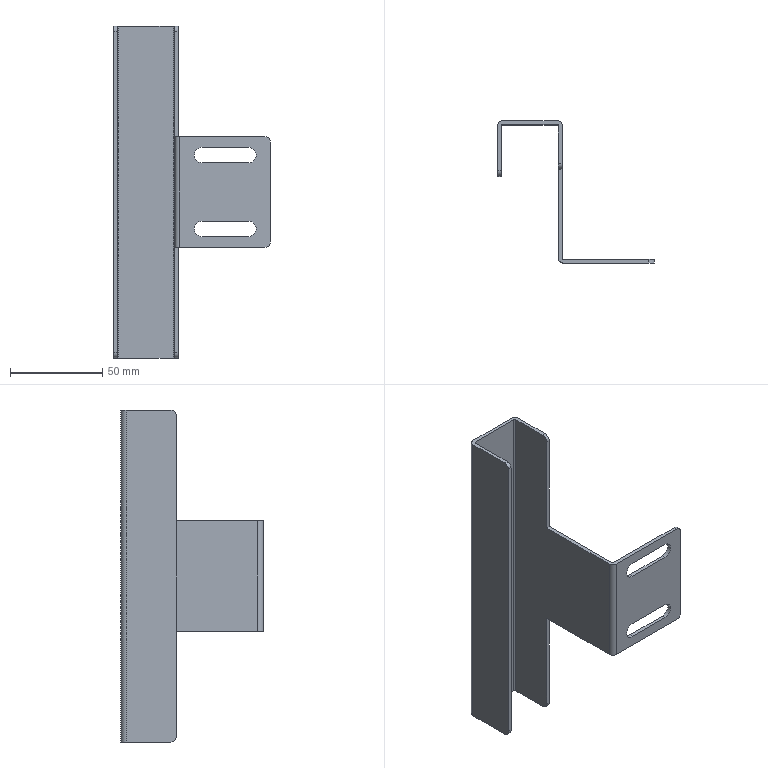Part | SolidWorks | features BaseBody 1 | 1 solid | 36 faces | box 85 x 77 x 180 mm | volume 41775 mm3 | plane 20 | cylinder 16 | commonest cylinder face diameters 6 x6 8.5 x4 1.473 x3 5.473 x3
STEP:
#1=CARTESIAN_POINT('',(35.,-23.255,-90.));
#2=VERTEX_POINT('',#1);
#3=CARTESIAN_POINT('',(35.,-2.737,-90.));
#4=VERTEX_POINT('',#3);
#5=CARTESIAN_POINT('',(35.,0.,-90.));
#6=DIRECTION('',(0.,1.,0.));
#7=VECTOR('',#6,1000.);
#8=LINE('',#5,#7);
#9=EDGE_CURVE('',#2,#4,#8,.T.);
#10=ORIENTED_EDGE('',*,*,#9,.T.);
#11=CARTESIAN_POINT('',(35.,-2.737,90.));
#12=VERTEX_POINT('',#11);
#13=CARTESIAN_POINT('',(35.,-2.737,90.));
#14=DIRECTION('',(0.,0.,1.));
#15=VECTOR('',#14,1000.);
#16=LINE('',#13,#15);
#17=EDGE_CURVE('',#4,#12,#16,.T.);
#18=ORIENTED_EDGE('',*,*,#17,.T.);
#19=CARTESIAN_POINT('',(35.,-23.255,90.));
#20=VERTEX_POINT('',#19);
#21=CARTESIAN_POINT('',(35.,0.,90.));
#22=DIRECTION('',(0.,-1.,0.));
#23=VECTOR('',#22,1000.);
#24=LINE('',#21,#23);
#25=EDGE_CURVE('',#12,#20,#24,.T.);
#26=ORIENTED_EDGE('',*,*,#25,.T.);
#27=CARTESIAN_POINT('',(35.,-26.255,87.));
#28=VERTEX_POINT('',#27);
#29=CARTESIAN_POINT('',(35.,-23.255,87.));
#30=DIRECTION('',(1.,0.,0.));
#31=DIRECTION('',(0.,0.,1.));
#32=AXIS2_PLACEMENT_3D('',#29,#30,#31);
#33=CIRCLE('',#32,3.);
#34=EDGE_CURVE('',#20,#28,#33,.T.);
#35=ORIENTED_EDGE('',*,*,#34,.T.);
#36=CARTESIAN_POINT('',(35.,-26.255,30.));
#37=VERTEX_POINT('',#36);
#38=CARTESIAN_POINT('',(35.,-26.255,90.));
#39=DIRECTION('',(0.,0.,-1.));
#40=VECTOR('',#39,1000.);
#41=LINE('',#38,#40);
#42=EDGE_CURVE('',#28,#37,#41,.T.);
#43=ORIENTED_EDGE('',*,*,#42,.T.);
#44=CARTESIAN_POINT('',(35.,-74.263,30.));
#45=VERTEX_POINT('',#44);
#46=CARTESIAN_POINT('',(35.,0.,30.));
#47=DIRECTION('',(0.,-1.,0.));
#48=VECTOR('',#47,1000.);
#49=LINE('',#46,#48);
#50=EDGE_CURVE('',#37,#45,#49,.T.);
#51=ORIENTED_EDGE('',*,*,#50,.T.);
#52=CARTESIAN_POINT('',(35.,-74.263,-30.));
#53=VERTEX_POINT('',#52);
#54=CARTESIAN_POINT('',(35.,-74.263,90.));
#55=DIRECTION('',(0.,0.,-1.));
#56=VECTOR('',#55,1000.);
#57=LINE('',#54,#56);
#58=EDGE_CURVE('',#45,#53,#57,.T.);
#59=ORIENTED_EDGE('',*,*,#58,.T.);
#60=CARTESIAN_POINT('',(35.,-26.255,-30.));
#61=VERTEX_POINT('',#60);
#62=CARTESIAN_POINT('',(35.,0.,-30.));
#63=DIRECTION('',(0.,1.,0.));
#64=VECTOR('',#63,1000.);
#65=LINE('',#62,#64);
#66=EDGE_CURVE('',#53,#61,#65,.T.);
#67=ORIENTED_EDGE('',*,*,#66,.T.);
#68=CARTESIAN_POINT('',(35.,-26.255,-87.));
#69=VERTEX_POINT('',#68);
#70=CARTESIAN_POINT('',(35.,-26.255,90.));
#71=DIRECTION('',(0.,0.,-1.));
#72=VECTOR('',#71,1000.);
#73=LINE('',#70,#72);
#74=EDGE_CURVE('',#61,#69,#73,.T.);
#75=ORIENTED_EDGE('',*,*,#74,.T.);
#76=CARTESIAN_POINT('',(35.,-23.255,-87.));
#77=DIRECTION('',(1.,0.,0.));
#78=DIRECTION('',(0.,0.,1.));
#79=AXIS2_PLACEMENT_3D('',#76,#77,#78);
#80=CIRCLE('',#79,3.);
#81=EDGE_CURVE('',#69,#2,#80,.T.);
#82=ORIENTED_EDGE('',*,*,#81,.T.);
#83=EDGE_LOOP('',(#10,#18,#26,#35,#43,#51,#59,#67,#75,#82));
#84=FACE_OUTER_BOUND('',#83,.T.);
#85=CARTESIAN_POINT('',(35.,0.,90.));
#86=DIRECTION('',(1.,0.,0.));
#87=DIRECTION('',(0.,0.,-1.));
#88=AXIS2_PLACEMENT_3D('',#85,#86,#87);
#89=PLANE('',#88);
#90=ADVANCED_FACE('',(#84),#89,.T.);
#91=CARTESIAN_POINT('',(32.263,0.,90.));
#92=VERTEX_POINT('',#91);
#93=CARTESIAN_POINT('',(32.263,-2.737,90.));
#94=DIRECTION('',(0.,0.,-1.));
#95=DIRECTION('',(-1.,0.,0.));
#96=AXIS2_PLACEMENT_3D('',#93,#94,#95);
#97=CIRCLE('',#96,2.737);
#98=EDGE_CURVE('',#92,#12,#97,.T.);
#99=ORIENTED_EDGE('',*,*,#98,.T.);
#100=ORIENTED_EDGE('',*,*,#17,.F.);
#101=CARTESIAN_POINT('',(32.263,0.,-90.));
#102=VERTEX_POINT('',#101);
#103=CARTESIAN_POINT('',(32.263,-2.737,-90.));
#104=DIRECTION('',(0.,0.,1.));
#105=DIRECTION('',(-1.,0.,0.));
#106=AXIS2_PLACEMENT_3D('',#103,#104,#105);
#107=CIRCLE('',#106,2.737);
#108=EDGE_CURVE('',#4,#102,#107,.T.);
#109=ORIENTED_EDGE('',*,*,#108,.T.);
#110=CARTESIAN_POINT('',(32.263,0.,90.));
#111=DIRECTION('',(0.,0.,1.));
#112=VECTOR('',#111,1000.);
#113=LINE('',#110,#112);
#114=EDGE_CURVE('',#102,#92,#113,.T.);
#115=ORIENTED_EDGE('',*,*,#114,.T.);
#116=EDGE_LOOP('',(#99,#100,#109,#115));
#117=FACE_OUTER_BOUND('',#116,.T.);
#118=CARTESIAN_POINT('',(32.263,-2.737,90.));
#119=DIRECTION('',(0.,0.,-1.));
#120=DIRECTION('',(-1.,0.,0.));
#121=AXIS2_PLACEMENT_3D('',#118,#119,#120);
#122=CYLINDRICAL_SURFACE('',#121,2.737);
#123=ADVANCED_FACE('',(#117),#122,.T.);
#124=CARTESIAN_POINT('',(33.,-23.255,-90.));
#125=VERTEX_POINT('',#124);
#126=CARTESIAN_POINT('',(33.,-2.737,-90.));
#127=VERTEX_POINT('',#126);
#128=CARTESIAN_POINT('',(33.,-77.,-90.));
#129=DIRECTION('',(0.,1.,0.));
#130=VECTOR('',#129,1000.);
#131=LINE('',#128,#130);
#132=EDGE_CURVE('',#125,#127,#131,.T.);
#133=ORIENTED_EDGE('',*,*,#132,.T.);
#134=CARTESIAN_POINT('',(32.263,-2.,-90.));
#135=VERTEX_POINT('',#134);
#136=CARTESIAN_POINT('',(32.263,-2.737,-90.));
#137=DIRECTION('',(0.,0.,1.));
#138=DIRECTION('',(-1.,0.,0.));
#139=AXIS2_PLACEMENT_3D('',#136,#137,#138);
#140=CIRCLE('',#139,0.7366);
#141=EDGE_CURVE('',#127,#135,#140,.T.);
#142=ORIENTED_EDGE('',*,*,#141,.T.);
#143=CARTESIAN_POINT('',(2.737,-2.,-90.));
#144=VERTEX_POINT('',#143);
#145=CARTESIAN_POINT('',(33.,-2.,-90.));
#146=DIRECTION('',(-1.,0.,0.));
#147=VECTOR('',#146,1000.);
#148=LINE('',#145,#147);
#149=EDGE_CURVE('',#135,#144,#148,.T.);
#150=ORIENTED_EDGE('',*,*,#149,.T.);
#151=CARTESIAN_POINT('',(2.,-2.737,-90.));
#152=VERTEX_POINT('',#151);
#153=CARTESIAN_POINT('',(2.737,-2.737,-90.));
#154=DIRECTION('',(0.,0.,1.));
#155=DIRECTION('',(-1.,0.,0.));
#156=AXIS2_PLACEMENT_3D('',#153,#154,#155);
#157=CIRCLE('',#156,0.7366);
#158=EDGE_CURVE('',#144,#152,#157,.T.);
#159=ORIENTED_EDGE('',*,*,#158,.T.);
#160=CARTESIAN_POINT('',(2.,-27.,-90.));
#161=VERTEX_POINT('',#160);
#162=CARTESIAN_POINT('',(2.,-2.,-90.));
#163=DIRECTION('',(0.,-1.,0.));
#164=VECTOR('',#163,1000.);
#165=LINE('',#162,#164);
#166=EDGE_CURVE('',#152,#161,#165,.T.);
#167=ORIENTED_EDGE('',*,*,#166,.T.);
#168=CARTESIAN_POINT('',(0.,-27.,-90.));
#169=VERTEX_POINT('',#168);
#170=CARTESIAN_POINT('',(2.737,-27.,-90.));
#171=DIRECTION('',(1.,0.,0.));
#172=VECTOR('',#171,1000.);
#173=LINE('',#170,#172);
#174=EDGE_CURVE('',#169,#161,#173,.T.);
#175=ORIENTED_EDGE('',*,*,#174,.F.);
#176=CARTESIAN_POINT('',(0.,-2.737,-90.));
#177=VERTEX_POINT('',#176);
#178=CARTESIAN_POINT('',(0.,-30.,-90.));
#179=DIRECTION('',(0.,-1.,0.));
#180=VECTOR('',#179,1000.);
#181=LINE('',#178,#180);
#182=EDGE_CURVE('',#177,#169,#181,.T.);
#183=ORIENTED_EDGE('',*,*,#182,.F.);
#184=CARTESIAN_POINT('',(2.737,0.,-90.));
#185=VERTEX_POINT('',#184);
#186=CARTESIAN_POINT('',(2.737,-2.737,-90.));
#187=DIRECTION('',(0.,0.,1.));
#188=DIRECTION('',(-1.,0.,0.));
#189=AXIS2_PLACEMENT_3D('',#186,#187,#188);
#190=CIRCLE('',#189,2.737);
#191=EDGE_CURVE('',#185,#177,#190,.T.);
#192=ORIENTED_EDGE('',*,*,#191,.F.);
#193=CARTESIAN_POINT('',(0.,0.,-90.));
#194=DIRECTION('',(-1.,0.,0.));
#195=VECTOR('',#194,1000.);
#196=LINE('',#193,#195);
#197=EDGE_CURVE('',#102,#185,#196,.T.);
#198=ORIENTED_EDGE('',*,*,#197,.F.);
#199=ORIENTED_EDGE('',*,*,#108,.F.);
#200=ORIENTED_EDGE('',*,*,#9,.F.);
#201=CARTESIAN_POINT('',(35.737,-23.255,-90.));
#202=DIRECTION('',(-1.,0.,0.));
#203=VECTOR('',#202,1000.);
#204=LINE('',#201,#203);
#205=EDGE_CURVE('',#2,#125,#204,.T.);
#206=ORIENTED_EDGE('',*,*,#205,.T.);
#207=EDGE_LOOP('',(#133,#142,#150,#159,#167,#175,#183,#192,#198,#199,#200,#206));
#208=FACE_OUTER_BOUND('',#207,.T.);
#209=CARTESIAN_POINT('',(35.737,-77.,-90.));
#210=DIRECTION('',(0.,0.,-1.));
#211=DIRECTION('',(-1.,0.,0.));
#212=AXIS2_PLACEMENT_3D('',#209,#210,#211);
#213=PLANE('',#212);
#214=ADVANCED_FACE('',(#208),#213,.T.);
#215=ORIENTED_EDGE('',*,*,#81,.F.);
#216=CARTESIAN_POINT('',(33.,-26.255,-87.));
#217=VERTEX_POINT('',#216);
#218=CARTESIAN_POINT('',(25.,-26.255,-87.));
#219=DIRECTION('',(-1.,0.,0.));
#220=VECTOR('',#219,1000.);
#221=LINE('',#218,#220);
#222=EDGE_CURVE('',#69,#217,#221,.T.);
#223=ORIENTED_EDGE('',*,*,#222,.T.);
#224=CARTESIAN_POINT('',(33.,-23.255,-87.));
#225=DIRECTION('',(1.,0.,0.));
#226=DIRECTION('',(0.,0.,1.));
#227=AXIS2_PLACEMENT_3D('',#224,#225,#226);
#228=CIRCLE('',#227,3.);
#229=EDGE_CURVE('',#217,#125,#228,.T.);
#230=ORIENTED_EDGE('',*,*,#229,.T.);
#231=ORIENTED_EDGE('',*,*,#205,.F.);
#232=EDGE_LOOP('',(#215,#223,#230,#231));
#233=FACE_OUTER_BOUND('',#232,.T.);
#234=CARTESIAN_POINT('',(25.,-23.255,-87.));
#235=DIRECTION('',(-1.,0.,0.));
#236=DIRECTION('',(0.,0.,1.));
#237=AXIS2_PLACEMENT_3D('',#234,#235,#236);
#238=CYLINDRICAL_SURFACE('',#237,3.);
#239=ADVANCED_FACE('',(#233),#238,.T.);
#240=ORIENTED_EDGE('',*,*,#222,.F.);
#241=ORIENTED_EDGE('',*,*,#74,.F.);
#242=CARTESIAN_POINT('',(33.,-26.255,-30.));
#243=VERTEX_POINT('',#242);
#244=CARTESIAN_POINT('',(25.,-26.255,-30.));
#245=DIRECTION('',(1.,0.,0.));
#246=VECTOR('',#245,1000.);
#247=LINE('',#244,#246);
#248=EDGE_CURVE('',#243,#61,#247,.T.);
#249=ORIENTED_EDGE('',*,*,#248,.F.);
#250=CARTESIAN_POINT('',(33.,-26.255,-90.));
#251=DIRECTION('',(0.,0.,1.));
#252=VECTOR('',#251,1000.);
#253=LINE('',#250,#252);
#254=EDGE_CURVE('',#217,#243,#253,.T.);
#255=ORIENTED_EDGE('',*,*,#254,.F.);
#256=EDGE_LOOP('',(#240,#241,#249,#255));
#257=FACE_OUTER_BOUND('',#256,.T.);
#258=CARTESIAN_POINT('',(25.,-26.255,-90.));
#259=DIRECTION('',(0.,1.,0.));
#260=DIRECTION('',(0.,0.,1.));
#261=AXIS2_PLACEMENT_3D('',#258,#259,#260);
#262=PLANE('',#261);
#263=ADVANCED_FACE('',(#257),#262,.F.);
#264=CARTESIAN_POINT('',(33.,-74.263,-30.));
#265=VERTEX_POINT('',#264);
#266=CARTESIAN_POINT('',(33.,-126.255,-30.));
#267=DIRECTION('',(0.,-1.,0.));
#268=VECTOR('',#267,1000.);
#269=LINE('',#266,#268);
#270=EDGE_CURVE('',#243,#265,#269,.T.);
#271=ORIENTED_EDGE('',*,*,#270,.F.);
#272=ORIENTED_EDGE('',*,*,#248,.T.);
#273=ORIENTED_EDGE('',*,*,#66,.F.);
#274=CARTESIAN_POINT('',(35.737,-75.,-30.));
#275=VERTEX_POINT('',#274);
#276=CARTESIAN_POINT('',(35.737,-74.263,-30.));
#277=DIRECTION('',(0.,0.,1.));
#278=DIRECTION('',(-1.,0.,0.));
#279=AXIS2_PLACEMENT_3D('',#276,#277,#278);
#280=CIRCLE('',#279,0.7366);
#281=EDGE_CURVE('',#53,#275,#280,.T.);
#282=ORIENTED_EDGE('',*,*,#281,.T.);
#283=CARTESIAN_POINT('',(82.,-75.,-30.));
#284=VERTEX_POINT('',#283);
#285=CARTESIAN_POINT('',(35.,-75.,-30.));
#286=DIRECTION('',(-1.,0.,0.));
#287=VECTOR('',#286,1000.);
#288=LINE('',#285,#287);
#289=EDGE_CURVE('',#284,#275,#288,.T.);
#290=ORIENTED_EDGE('',*,*,#289,.F.);
#291=CARTESIAN_POINT('',(82.,-77.,-30.));
#292=VERTEX_POINT('',#291);
#293=CARTESIAN_POINT('',(82.,-85.,-30.));
#294=DIRECTION('',(0.,1.,0.));
#295=VECTOR('',#294,1000.);
#296=LINE('',#293,#295);
#297=EDGE_CURVE('',#292,#284,#296,.T.);
#298=ORIENTED_EDGE('',*,*,#297,.F.);
#299=CARTESIAN_POINT('',(35.737,-77.,-30.));
#300=VERTEX_POINT('',#299);
#301=CARTESIAN_POINT('',(85.,-77.,-30.));
#302=DIRECTION('',(1.,0.,0.));
#303=VECTOR('',#302,1000.);
#304=LINE('',#301,#303);
#305=EDGE_CURVE('',#300,#292,#304,.T.);
#306=ORIENTED_EDGE('',*,*,#305,.F.);
#307=CARTESIAN_POINT('',(35.737,-74.263,-30.));
#308=DIRECTION('',(0.,0.,1.));
#309=DIRECTION('',(-1.,0.,0.));
#310=AXIS2_PLACEMENT_3D('',#307,#308,#309);
#311=CIRCLE('',#310,2.737);
#312=EDGE_CURVE('',#265,#300,#311,.T.);
#313=ORIENTED_EDGE('',*,*,#312,.F.);
#314=EDGE_LOOP('',(#271,#272,#273,#282,#290,#298,#306,#313));
#315=FACE_OUTER_BOUND('',#314,.T.);
#316=CARTESIAN_POINT('',(25.,-126.255,-30.));
#317=DIRECTION('',(0.,0.,1.));
#318=DIRECTION('',(1.,0.,0.));
#319=AXIS2_PLACEMENT_3D('',#316,#317,#318);
#320=PLANE('',#319);
#321=ADVANCED_FACE('',(#315),#320,.F.);
#322=ORIENTED_EDGE('',*,*,#58,.F.);
#323=CARTESIAN_POINT('',(35.737,-75.,30.));
#324=VERTEX_POINT('',#323);
#325=CARTESIAN_POINT('',(35.737,-74.263,30.));
#326=DIRECTION('',(0.,0.,1.));
#327=DIRECTION('',(-1.,0.,0.));
#328=AXIS2_PLACEMENT_3D('',#325,#326,#327);
#329=CIRCLE('',#328,0.7366);
#330=EDGE_CURVE('',#45,#324,#329,.T.);
#331=ORIENTED_EDGE('',*,*,#330,.T.);
#332=CARTESIAN_POINT('',(35.737,-75.,60.095));
#333=DIRECTION('',(0.,0.,1.));
#334=VECTOR('',#333,1000.);
#335=LINE('',#332,#334);
#336=EDGE_CURVE('',#275,#324,#335,.T.);
#337=ORIENTED_EDGE('',*,*,#336,.F.);
#338=ORIENTED_EDGE('',*,*,#281,.F.);
#339=EDGE_LOOP('',(#322,#331,#337,#338));
#340=FACE_OUTER_BOUND('',#339,.T.);
#341=CARTESIAN_POINT('',(35.737,-74.263,60.095));
#342=DIRECTION('',(0.,0.,-1.));
#343=DIRECTION('',(-1.,0.,0.));
#344=AXIS2_PLACEMENT_3D('',#341,#342,#343);
#345=CYLINDRICAL_SURFACE('',#344,0.7366);
#346=ADVANCED_FACE('',(#340),#345,.F.);
#347=ORIENTED_EDGE('',*,*,#50,.F.);
#348=CARTESIAN_POINT('',(33.,-26.255,30.));
#349=VERTEX_POINT('',#348);
#350=CARTESIAN_POINT('',(25.,-26.255,30.));
#351=DIRECTION('',(1.,0.,0.));
#352=VECTOR('',#351,1000.);
#353=LINE('',#350,#352);
#354=EDGE_CURVE('',#349,#37,#353,.T.);
#355=ORIENTED_EDGE('',*,*,#354,.F.);
#356=CARTESIAN_POINT('',(33.,-74.263,30.));
#357=VERTEX_POINT('',#356);
#358=CARTESIAN_POINT('',(33.,-126.255,30.));
#359=DIRECTION('',(0.,1.,0.));
#360=VECTOR('',#359,1000.);
#361=LINE('',#358,#360);
#362=EDGE_CURVE('',#357,#349,#361,.T.);
#363=ORIENTED_EDGE('',*,*,#362,.F.);
#364=CARTESIAN_POINT('',(35.737,-77.,30.));
#365=VERTEX_POINT('',#364);
#366=CARTESIAN_POINT('',(35.737,-74.263,30.));
#367=DIRECTION('',(0.,0.,-1.));
#368=DIRECTION('',(-1.,0.,0.));
#369=AXIS2_PLACEMENT_3D('',#366,#367,#368);
#370=CIRCLE('',#369,2.737);
#371=EDGE_CURVE('',#365,#357,#370,.T.);
#372=ORIENTED_EDGE('',*,*,#371,.F.);
#373=CARTESIAN_POINT('',(82.,-77.,30.));
#374=VERTEX_POINT('',#373);
#375=CARTESIAN_POINT('',(85.,-77.,30.));
#376=DIRECTION('',(-1.,0.,0.));
#377=VECTOR('',#376,1000.);
#378=LINE('',#375,#377);
#379=EDGE_CURVE('',#374,#365,#378,.T.);
#380=ORIENTED_EDGE('',*,*,#379,.F.);
#381=CARTESIAN_POINT('',(82.,-75.,30.));
#382=VERTEX_POINT('',#381);
#383=CARTESIAN_POINT('',(82.,-85.,30.));
#384=DIRECTION('',(0.,-1.,0.));
#385=VECTOR('',#384,1000.);
#386=LINE('',#383,#385);
#387=EDGE_CURVE('',#382,#374,#386,.T.);
#388=ORIENTED_EDGE('',*,*,#387,.F.);
#389=CARTESIAN_POINT('',(35.,-75.,30.));
#390=DIRECTION('',(1.,0.,0.));
#391=VECTOR('',#390,1000.);
#392=LINE('',#389,#391);
#393=EDGE_CURVE('',#324,#382,#392,.T.);
#394=ORIENTED_EDGE('',*,*,#393,.F.);
#395=ORIENTED_EDGE('',*,*,#330,.F.);
#396=EDGE_LOOP('',(#347,#355,#363,#372,#380,#388,#394,#395));
#397=FACE_OUTER_BOUND('',#396,.T.);
#398=CARTESIAN_POINT('',(25.,-126.255,30.));
#399=DIRECTION('',(0.,0.,-1.));
#400=DIRECTION('',(0.,1.,0.));
#401=AXIS2_PLACEMENT_3D('',#398,#399,#400);
#402=PLANE('',#401);
#403=ADVANCED_FACE('',(#397),#402,.F.);
#404=CARTESIAN_POINT('',(33.,-26.255,87.));
#405=VERTEX_POINT('',#404);
#406=CARTESIAN_POINT('',(25.,-26.255,87.));
#407=DIRECTION('',(1.,0.,0.));
#408=VECTOR('',#407,1000.);
#409=LINE('',#406,#408);
#410=EDGE_CURVE('',#405,#28,#409,.T.);
#411=ORIENTED_EDGE('',*,*,#410,.F.);
#412=CARTESIAN_POINT('',(33.,-26.255,90.));
#413=DIRECTION('',(0.,0.,1.));
#414=VECTOR('',#413,1000.);
#415=LINE('',#412,#414);
#416=EDGE_CURVE('',#349,#405,#415,.T.);
#417=ORIENTED_EDGE('',*,*,#416,.F.);
#418=ORIENTED_EDGE('',*,*,#354,.T.);
#419=ORIENTED_EDGE('',*,*,#42,.F.);
#420=EDGE_LOOP('',(#411,#417,#418,#419));
#421=FACE_OUTER_BOUND('',#420,.T.);
#422=CARTESIAN_POINT('',(25.,-26.255,90.));
#423=DIRECTION('',(0.,1.,0.));
#424=DIRECTION('',(0.,0.,1.));
#425=AXIS2_PLACEMENT_3D('',#422,#423,#424);
#426=PLANE('',#425);
#427=ADVANCED_FACE('',(#421),#426,.F.);
#428=ORIENTED_EDGE('',*,*,#34,.F.);
#429=CARTESIAN_POINT('',(33.,-23.255,90.));
#430=VERTEX_POINT('',#429);
#431=CARTESIAN_POINT('',(32.263,-23.255,90.));
#432=DIRECTION('',(-1.,0.,0.));
#433=VECTOR('',#432,1000.);
#434=LINE('',#431,#433);
#435=EDGE_CURVE('',#20,#430,#434,.T.);
#436=ORIENTED_EDGE('',*,*,#435,.T.);
#437=CARTESIAN_POINT('',(33.,-23.255,87.));
#438=DIRECTION('',(1.,0.,0.));
#439=DIRECTION('',(0.,0.,1.));
#440=AXIS2_PLACEMENT_3D('',#437,#438,#439);
#441=CIRCLE('',#440,3.);
#442=EDGE_CURVE('',#430,#405,#441,.T.);
#443=ORIENTED_EDGE('',*,*,#442,.T.);
#444=ORIENTED_EDGE('',*,*,#410,.T.);
#445=EDGE_LOOP('',(#428,#436,#443,#444));
#446=FACE_OUTER_BOUND('',#445,.T.);
#447=CARTESIAN_POINT('',(32.263,-23.255,87.));
#448=DIRECTION('',(-1.,0.,0.));
#449=DIRECTION('',(0.,0.,1.));
#450=AXIS2_PLACEMENT_3D('',#447,#448,#449);
#451=CYLINDRICAL_SURFACE('',#450,3.);
#452=ADVANCED_FACE('',(#446),#451,.T.);
#453=ORIENTED_EDGE('',*,*,#25,.F.);
#454=ORIENTED_EDGE('',*,*,#98,.F.);
#455=CARTESIAN_POINT('',(2.737,0.,90.));
#456=VERTEX_POINT('',#455);
#457=CARTESIAN_POINT('',(0.,0.,90.));
#458=DIRECTION('',(1.,0.,0.));
#459=VECTOR('',#458,1000.);
#460=LINE('',#457,#459);
#461=EDGE_CURVE('',#456,#92,#460,.T.);
#462=ORIENTED_EDGE('',*,*,#461,.F.);
#463=CARTESIAN_POINT('',(0.,-2.737,90.));
#464=VERTEX_POINT('',#463);
#465=CARTESIAN_POINT('',(2.737,-2.737,90.));
#466=DIRECTION('',(0.,0.,-1.));
#467=DIRECTION('',(-1.,0.,0.));
#468=AXIS2_PLACEMENT_3D('',#465,#466,#467);
#469=CIRCLE('',#468,2.737);
#470=EDGE_CURVE('',#464,#456,#469,.T.);
#471=ORIENTED_EDGE('',*,*,#470,.F.);
#472=CARTESIAN_POINT('',(0.,-27.,90.));
#473=VERTEX_POINT('',#472);
#474=CARTESIAN_POINT('',(0.,-30.,90.));
#475=DIRECTION('',(0.,1.,0.));
#476=VECTOR('',#475,1000.);
#477=LINE('',#474,#476);
#478=EDGE_CURVE('',#473,#464,#477,.T.);
#479=ORIENTED_EDGE('',*,*,#478,.F.);
#480=CARTESIAN_POINT('',(2.,-27.,90.));
#481=VERTEX_POINT('',#480);
#482=CARTESIAN_POINT('',(35.737,-27.,90.));
#483=DIRECTION('',(-1.,0.,0.));
#484=VECTOR('',#483,1000.);
#485=LINE('',#482,#484);
#486=EDGE_CURVE('',#481,#473,#485,.T.);
#487=ORIENTED_EDGE('',*,*,#486,.F.);
#488=CARTESIAN_POINT('',(2.,-2.737,90.));
#489=VERTEX_POINT('',#488);
#490=CARTESIAN_POINT('',(2.,-74.263,90.));
#491=DIRECTION('',(0.,-1.,0.));
#492=VECTOR('',#491,1000.);
#493=LINE('',#490,#492);
#494=EDGE_CURVE('',#489,#481,#493,.T.);
#495=ORIENTED_EDGE('',*,*,#494,.F.);
#496=CARTESIAN_POINT('',(2.737,-2.,90.));
#497=VERTEX_POINT('',#496);
#498=CARTESIAN_POINT('',(2.737,-2.737,90.));
#499=DIRECTION('',(0.,0.,-1.));
#500=DIRECTION('',(-1.,0.,0.));
#501=AXIS2_PLACEMENT_3D('',#498,#499,#500);
#502=CIRCLE('',#501,0.7366);
#503=EDGE_CURVE('',#489,#497,#502,.T.);
#504=ORIENTED_EDGE('',*,*,#503,.T.);
#505=CARTESIAN_POINT('',(32.263,-2.,90.));
#506=VERTEX_POINT('',#505);
#507=CARTESIAN_POINT('',(2.,-2.,90.));
#508=DIRECTION('',(1.,0.,0.));
#509=VECTOR('',#508,1000.);
#510=LINE('',#507,#509);
#511=EDGE_CURVE('',#497,#506,#510,.T.);
#512=ORIENTED_EDGE('',*,*,#511,.T.);
#513=CARTESIAN_POINT('',(33.,-2.737,90.));
#514=VERTEX_POINT('',#513);
#515=CARTESIAN_POINT('',(32.263,-2.737,90.));
#516=DIRECTION('',(0.,0.,-1.));
#517=DIRECTION('',(-1.,0.,0.));
#518=AXIS2_PLACEMENT_3D('',#515,#516,#517);
#519=CIRCLE('',#518,0.7366);
#520=EDGE_CURVE('',#506,#514,#519,.T.);
#521=ORIENTED_EDGE('',*,*,#520,.T.);
#522=CARTESIAN_POINT('',(33.,-2.,90.));
#523=DIRECTION('',(0.,-1.,0.));
#524=VECTOR('',#523,1000.);
#525=LINE('',#522,#524);
#526=EDGE_CURVE('',#514,#430,#525,.T.);
#527=ORIENTED_EDGE('',*,*,#526,.T.);
#528=ORIENTED_EDGE('',*,*,#435,.F.);
#529=EDGE_LOOP('',(#453,#454,#462,#471,#479,#487,#495,#504,#512,#521,#527,#528));
#530=FACE_OUTER_BOUND('',#529,.T.);
#531=CARTESIAN_POINT('',(32.263,-2.,90.));
#532=DIRECTION('',(0.,0.,1.));
#533=DIRECTION('',(1.,0.,0.));
#534=AXIS2_PLACEMENT_3D('',#531,#532,#533);
#535=PLANE('',#534);
#536=ADVANCED_FACE('',(#530),#535,.T.);
#537=ORIENTED_EDGE('',*,*,#461,.T.);
#538=ORIENTED_EDGE('',*,*,#114,.F.);
#539=ORIENTED_EDGE('',*,*,#197,.T.);
#540=CARTESIAN_POINT('',(2.737,0.,90.));
#541=DIRECTION('',(0.,0.,1.));
#542=VECTOR('',#541,1000.);
#543=LINE('',#540,#542);
#544=EDGE_CURVE('',#185,#456,#543,.T.);
#545=ORIENTED_EDGE('',*,*,#544,.T.);
#546=EDGE_LOOP('',(#537,#538,#539,#545));
#547=FACE_OUTER_BOUND('',#546,.T.);
#548=CARTESIAN_POINT('',(0.,0.,90.));
#549=DIRECTION('',(0.,1.,0.));
#550=DIRECTION('',(0.,0.,1.));
#551=AXIS2_PLACEMENT_3D('',#548,#549,#550);
#552=PLANE('',#551);
#553=ADVANCED_FACE('',(#547),#552,.T.);
#554=ORIENTED_EDGE('',*,*,#442,.F.);
#555=ORIENTED_EDGE('',*,*,#526,.F.);
#556=CARTESIAN_POINT('',(33.,-2.737,90.));
#557=DIRECTION('',(0.,0.,1.));
#558=VECTOR('',#557,1000.);
#559=LINE('',#556,#558);
#560=EDGE_CURVE('',#127,#514,#559,.T.);
#561=ORIENTED_EDGE('',*,*,#560,.F.);
#562=ORIENTED_EDGE('',*,*,#132,.F.);
#563=ORIENTED_EDGE('',*,*,#229,.F.);
#564=ORIENTED_EDGE('',*,*,#254,.T.);
#565=ORIENTED_EDGE('',*,*,#270,.T.);
#566=CARTESIAN_POINT('',(33.,-74.263,90.));
#567=DIRECTION('',(0.,0.,-1.));
#568=VECTOR('',#567,1000.);
#569=LINE('',#566,#568);
#570=EDGE_CURVE('',#357,#265,#569,.T.);
#571=ORIENTED_EDGE('',*,*,#570,.F.);
#572=ORIENTED_EDGE('',*,*,#362,.T.);
#573=ORIENTED_EDGE('',*,*,#416,.T.);
#574=EDGE_LOOP('',(#554,#555,#561,#562,#563,#564,#565,#571,#572,#573));
#575=FACE_OUTER_BOUND('',#574,.T.);
#576=CARTESIAN_POINT('',(33.,0.,90.));
#577=DIRECTION('',(1.,0.,0.));
#578=DIRECTION('',(0.,0.,-1.));
#579=AXIS2_PLACEMENT_3D('',#576,#577,#578);
#580=PLANE('',#579);
#581=ADVANCED_FACE('',(#575),#580,.F.);
#582=ORIENTED_EDGE('',*,*,#393,.T.);
#583=CARTESIAN_POINT('',(85.,-75.,27.));
#584=VERTEX_POINT('',#583);
#585=CARTESIAN_POINT('',(82.,-75.,27.));
#586=DIRECTION('',(0.,1.,0.));
#587=DIRECTION('',(0.,0.,-1.));
#588=AXIS2_PLACEMENT_3D('',#585,#586,#587);
#589=CIRCLE('',#588,3.);
#590=EDGE_CURVE('',#382,#584,#589,.T.);
#591=ORIENTED_EDGE('',*,*,#590,.T.);
#592=CARTESIAN_POINT('',(85.,-75.,-27.));
#593=VERTEX_POINT('',#592);
#594=CARTESIAN_POINT('',(85.,-75.,90.));
#595=DIRECTION('',(0.,0.,-1.));
#596=VECTOR('',#595,1000.);
#597=LINE('',#594,#596);
#598=EDGE_CURVE('',#584,#593,#597,.T.);
#599=ORIENTED_EDGE('',*,*,#598,.T.);
#600=CARTESIAN_POINT('',(82.,-75.,-27.));
#601=DIRECTION('',(0.,1.,0.));
#602=DIRECTION('',(0.,0.,-1.));
#603=AXIS2_PLACEMENT_3D('',#600,#601,#602);
#604=CIRCLE('',#603,3.);
#605=EDGE_CURVE('',#593,#284,#604,.T.);
#606=ORIENTED_EDGE('',*,*,#605,.T.);
#607=ORIENTED_EDGE('',*,*,#289,.T.);
#608=ORIENTED_EDGE('',*,*,#336,.T.);
#609=EDGE_LOOP('',(#582,#591,#599,#606,#607,#608));
#610=FACE_OUTER_BOUND('',#609,.T.);
#611=CARTESIAN_POINT('',(73.,-75.,15.75));
#612=VERTEX_POINT('',#611);
#613=CARTESIAN_POINT('',(73.,-75.,24.25));
#614=VERTEX_POINT('',#613);
#615=CARTESIAN_POINT('',(73.,-75.,20.));
#616=DIRECTION('',(0.,-1.,0.));
#617=DIRECTION('',(0.,0.,1.));
#618=AXIS2_PLACEMENT_3D('',#615,#616,#617);
#619=CIRCLE('',#618,4.25);
#620=EDGE_CURVE('',#612,#614,#619,.T.);
#621=ORIENTED_EDGE('',*,*,#620,.T.);
#622=CARTESIAN_POINT('',(48.,-75.,24.25));
#623=VERTEX_POINT('',#622);
#624=CARTESIAN_POINT('',(35.,-75.,24.25));
#625=DIRECTION('',(-1.,0.,0.));
#626=VECTOR('',#625,1000.);
#627=LINE('',#624,#626);
#628=EDGE_CURVE('',#614,#623,#627,.T.);
#629=ORIENTED_EDGE('',*,*,#628,.T.);
#630=CARTESIAN_POINT('',(48.,-75.,15.75));
#631=VERTEX_POINT('',#630);
#632=CARTESIAN_POINT('',(48.,-75.,20.));
#633=DIRECTION('',(0.,-1.,0.));
#634=DIRECTION('',(0.,0.,1.));
#635=AXIS2_PLACEMENT_3D('',#632,#633,#634);
#636=CIRCLE('',#635,4.25);
#637=EDGE_CURVE('',#623,#631,#636,.T.);
#638=ORIENTED_EDGE('',*,*,#637,.T.);
#639=CARTESIAN_POINT('',(35.,-75.,15.75));
#640=DIRECTION('',(1.,0.,0.));
#641=VECTOR('',#640,1000.);
#642=LINE('',#639,#641);
#643=EDGE_CURVE('',#631,#612,#642,.T.);
#644=ORIENTED_EDGE('',*,*,#643,.T.);
#645=EDGE_LOOP('',(#621,#629,#638,#644));
#646=FACE_BOUND('',#645,.T.);
#647=CARTESIAN_POINT('',(73.,-75.,-24.25));
#648=VERTEX_POINT('',#647);
#649=CARTESIAN_POINT('',(73.,-75.,-15.75));
#650=VERTEX_POINT('',#649);
#651=CARTESIAN_POINT('',(73.,-75.,-20.));
#652=DIRECTION('',(0.,-1.,0.));
#653=DIRECTION('',(0.,0.,1.));
#654=AXIS2_PLACEMENT_3D('',#651,#652,#653);
#655=CIRCLE('',#654,4.25);
#656=EDGE_CURVE('',#648,#650,#655,.T.);
#657=ORIENTED_EDGE('',*,*,#656,.T.);
#658=CARTESIAN_POINT('',(48.,-75.,-15.75));
#659=VERTEX_POINT('',#658);
#660=CARTESIAN_POINT('',(35.,-75.,-15.75));
#661=DIRECTION('',(-1.,0.,0.));
#662=VECTOR('',#661,1000.);
#663=LINE('',#660,#662);
#664=EDGE_CURVE('',#650,#659,#663,.T.);
#665=ORIENTED_EDGE('',*,*,#664,.T.);
#666=CARTESIAN_POINT('',(48.,-75.,-24.25));
#667=VERTEX_POINT('',#666);
#668=CARTESIAN_POINT('',(48.,-75.,-20.));
#669=DIRECTION('',(0.,-1.,0.));
#670=DIRECTION('',(0.,0.,1.));
#671=AXIS2_PLACEMENT_3D('',#668,#669,#670);
#672=CIRCLE('',#671,4.25);
#673=EDGE_CURVE('',#659,#667,#672,.T.);
#674=ORIENTED_EDGE('',*,*,#673,.T.);
#675=CARTESIAN_POINT('',(35.,-75.,-24.25));
#676=DIRECTION('',(1.,0.,0.));
#677=VECTOR('',#676,1000.);
#678=LINE('',#675,#677);
#679=EDGE_CURVE('',#667,#648,#678,.T.);
#680=ORIENTED_EDGE('',*,*,#679,.T.);
#681=EDGE_LOOP('',(#657,#665,#674,#680));
#682=FACE_BOUND('',#681,.T.);
#683=CARTESIAN_POINT('',(35.,-75.,90.));
#684=DIRECTION('',(0.,1.,0.));
#685=DIRECTION('',(0.,0.,1.));
#686=AXIS2_PLACEMENT_3D('',#683,#684,#685);
#687=PLANE('',#686);
#688=ADVANCED_FACE('',(#610,#646,#682),#687,.T.);
#689=ORIENTED_EDGE('',*,*,#470,.T.);
#690=ORIENTED_EDGE('',*,*,#544,.F.);
#691=ORIENTED_EDGE('',*,*,#191,.T.);
#692=CARTESIAN_POINT('',(0.,-2.737,90.));
#693=DIRECTION('',(0.,0.,1.));
#694=VECTOR('',#693,1000.);
#695=LINE('',#692,#694);
#696=EDGE_CURVE('',#177,#464,#695,.T.);
#697=ORIENTED_EDGE('',*,*,#696,.T.);
#698=EDGE_LOOP('',(#689,#690,#691,#697));
#699=FACE_OUTER_BOUND('',#698,.T.);
#700=CARTESIAN_POINT('',(2.737,-2.737,90.));
#701=DIRECTION('',(0.,0.,-1.));
#702=DIRECTION('',(-1.,0.,0.));
#703=AXIS2_PLACEMENT_3D('',#700,#701,#702);
#704=CYLINDRICAL_SURFACE('',#703,2.737);
#705=ADVANCED_FACE('',(#699),#704,.T.);
#706=ORIENTED_EDGE('',*,*,#560,.T.);
#707=ORIENTED_EDGE('',*,*,#520,.F.);
#708=CARTESIAN_POINT('',(32.263,-2.,90.));
#709=DIRECTION('',(0.,0.,1.));
#710=VECTOR('',#709,1000.);
#711=LINE('',#708,#710);
#712=EDGE_CURVE('',#135,#506,#711,.T.);
#713=ORIENTED_EDGE('',*,*,#712,.F.);
#714=ORIENTED_EDGE('',*,*,#141,.F.);
#715=EDGE_LOOP('',(#706,#707,#713,#714));
#716=FACE_OUTER_BOUND('',#715,.T.);
#717=CARTESIAN_POINT('',(32.263,-2.737,90.));
#718=DIRECTION('',(0.,0.,-1.));
#719=DIRECTION('',(-1.,0.,0.));
#720=AXIS2_PLACEMENT_3D('',#717,#718,#719);
#721=CYLINDRICAL_SURFACE('',#720,0.7366);
#722=ADVANCED_FACE('',(#716),#721,.F.);
#723=ORIENTED_EDGE('',*,*,#371,.T.);
#724=ORIENTED_EDGE('',*,*,#570,.T.);
#725=ORIENTED_EDGE('',*,*,#312,.T.);
#726=CARTESIAN_POINT('',(35.737,-77.,60.095));
#727=DIRECTION('',(0.,0.,1.));
#728=VECTOR('',#727,1000.);
#729=LINE('',#726,#728);
#730=EDGE_CURVE('',#300,#365,#729,.T.);
#731=ORIENTED_EDGE('',*,*,#730,.T.);
#732=EDGE_LOOP('',(#723,#724,#725,#731));
#733=FACE_OUTER_BOUND('',#732,.T.);
#734=CARTESIAN_POINT('',(35.737,-74.263,60.095));
#735=DIRECTION('',(0.,0.,-1.));
#736=DIRECTION('',(-1.,0.,0.));
#737=AXIS2_PLACEMENT_3D('',#734,#735,#736);
#738=CYLINDRICAL_SURFACE('',#737,2.737);
#739=ADVANCED_FACE('',(#733),#738,.T.);
#740=ORIENTED_EDGE('',*,*,#590,.F.);
#741=ORIENTED_EDGE('',*,*,#387,.T.);
#742=CARTESIAN_POINT('',(85.,-77.,27.));
#743=VERTEX_POINT('',#742);
#744=CARTESIAN_POINT('',(82.,-77.,27.));
#745=DIRECTION('',(0.,1.,0.));
#746=DIRECTION('',(0.,0.,-1.));
#747=AXIS2_PLACEMENT_3D('',#744,#745,#746);
#748=CIRCLE('',#747,3.);
#749=EDGE_CURVE('',#374,#743,#748,.T.);
#750=ORIENTED_EDGE('',*,*,#749,.T.);
#751=CARTESIAN_POINT('',(85.,-85.,27.));
#752=DIRECTION('',(0.,1.,0.));
#753=VECTOR('',#752,1000.);
#754=LINE('',#751,#753);
#755=EDGE_CURVE('',#743,#584,#754,.T.);
#756=ORIENTED_EDGE('',*,*,#755,.T.);
#757=EDGE_LOOP('',(#740,#741,#750,#756));
#758=FACE_OUTER_BOUND('',#757,.T.);
#759=CARTESIAN_POINT('',(82.,-85.,27.));
#760=DIRECTION('',(0.,-1.,0.));
#761=DIRECTION('',(0.,0.,-1.));
#762=AXIS2_PLACEMENT_3D('',#759,#760,#761);
#763=CYLINDRICAL_SURFACE('',#762,3.);
#764=ADVANCED_FACE('',(#758),#763,.T.);
#765=ORIENTED_EDGE('',*,*,#605,.F.);
#766=CARTESIAN_POINT('',(85.,-77.,-27.));
#767=VERTEX_POINT('',#766);
#768=CARTESIAN_POINT('',(85.,-75.,-27.));
#769=DIRECTION('',(0.,-1.,0.));
#770=VECTOR('',#769,1000.);
#771=LINE('',#768,#770);
#772=EDGE_CURVE('',#593,#767,#771,.T.);
#773=ORIENTED_EDGE('',*,*,#772,.T.);
#774=CARTESIAN_POINT('',(82.,-77.,-27.));
#775=DIRECTION('',(0.,1.,0.));
#776=DIRECTION('',(0.,0.,-1.));
#777=AXIS2_PLACEMENT_3D('',#774,#775,#776);
#778=CIRCLE('',#777,3.);
#779=EDGE_CURVE('',#767,#292,#778,.T.);
#780=ORIENTED_EDGE('',*,*,#779,.T.);
#781=ORIENTED_EDGE('',*,*,#297,.T.);
#782=EDGE_LOOP('',(#765,#773,#780,#781));
#783=FACE_OUTER_BOUND('',#782,.T.);
#784=CARTESIAN_POINT('',(82.,-75.,-27.));
#785=DIRECTION('',(0.,-1.,0.));
#786=DIRECTION('',(0.,0.,-1.));
#787=AXIS2_PLACEMENT_3D('',#784,#785,#786);
#788=CYLINDRICAL_SURFACE('',#787,3.);
#789=ADVANCED_FACE('',(#783),#788,.T.);
#790=ORIENTED_EDGE('',*,*,#598,.F.);
#791=ORIENTED_EDGE('',*,*,#755,.F.);
#792=CARTESIAN_POINT('',(85.,-77.,90.));
#793=DIRECTION('',(0.,0.,-1.));
#794=VECTOR('',#793,1000.);
#795=LINE('',#792,#794);
#796=EDGE_CURVE('',#743,#767,#795,.T.);
#797=ORIENTED_EDGE('',*,*,#796,.T.);
#798=ORIENTED_EDGE('',*,*,#772,.F.);
#799=EDGE_LOOP('',(#790,#791,#797,#798));
#800=FACE_OUTER_BOUND('',#799,.T.);
#801=CARTESIAN_POINT('',(85.,-75.,90.));
#802=DIRECTION('',(1.,0.,0.));
#803=DIRECTION('',(0.,0.,-1.));
#804=AXIS2_PLACEMENT_3D('',#801,#802,#803);
#805=PLANE('',#804);
#806=ADVANCED_FACE('',(#800),#805,.T.);
#807=ORIENTED_EDGE('',*,*,#628,.F.);
#808=CARTESIAN_POINT('',(73.,-77.,24.25));
#809=VERTEX_POINT('',#808);
#810=CARTESIAN_POINT('',(73.,-85.,24.25));
#811=DIRECTION('',(0.,1.,0.));
#812=VECTOR('',#811,1000.);
#813=LINE('',#810,#812);
#814=EDGE_CURVE('',#809,#614,#813,.T.);
#815=ORIENTED_EDGE('',*,*,#814,.F.);
#816=CARTESIAN_POINT('',(48.,-77.,24.25));
#817=VERTEX_POINT('',#816);
#818=CARTESIAN_POINT('',(48.,-77.,24.25));
#819=DIRECTION('',(1.,0.,0.));
#820=VECTOR('',#819,1000.);
#821=LINE('',#818,#820);
#822=EDGE_CURVE('',#817,#809,#821,.T.);
#823=ORIENTED_EDGE('',*,*,#822,.F.);
#824=CARTESIAN_POINT('',(48.,-85.,24.25));
#825=DIRECTION('',(0.,-1.,0.));
#826=VECTOR('',#825,1000.);
#827=LINE('',#824,#826);
#828=EDGE_CURVE('',#623,#817,#827,.T.);
#829=ORIENTED_EDGE('',*,*,#828,.F.);
#830=EDGE_LOOP('',(#807,#815,#823,#829));
#831=FACE_OUTER_BOUND('',#830,.T.);
#832=CARTESIAN_POINT('',(48.,-85.,24.25));
#833=DIRECTION('',(0.,0.,1.));
#834=DIRECTION('',(1.,0.,0.));
#835=AXIS2_PLACEMENT_3D('',#832,#833,#834);
#836=PLANE('',#835);
#837=ADVANCED_FACE('',(#831),#836,.F.);
#838=ORIENTED_EDGE('',*,*,#620,.F.);
#839=CARTESIAN_POINT('',(73.,-77.,15.75));
#840=VERTEX_POINT('',#839);
#841=CARTESIAN_POINT('',(73.,-85.,15.75));
#842=DIRECTION('',(0.,1.,0.));
#843=VECTOR('',#842,1000.);
#844=LINE('',#841,#843);
#845=EDGE_CURVE('',#840,#612,#844,.T.);
#846=ORIENTED_EDGE('',*,*,#845,.F.);
#847=CARTESIAN_POINT('',(73.,-77.,20.));
#848=DIRECTION('',(0.,1.,0.));
#849=DIRECTION('',(0.,0.,1.));
#850=AXIS2_PLACEMENT_3D('',#847,#848,#849);
#851=CIRCLE('',#850,4.25);
#852=EDGE_CURVE('',#809,#840,#851,.T.);
#853=ORIENTED_EDGE('',*,*,#852,.F.);
#854=ORIENTED_EDGE('',*,*,#814,.T.);
#855=EDGE_LOOP('',(#838,#846,#853,#854));
#856=FACE_OUTER_BOUND('',#855,.T.);
#857=CARTESIAN_POINT('',(73.,-85.,20.));
#858=DIRECTION('',(0.,1.,0.));
#859=DIRECTION('',(0.,0.,1.));
#860=AXIS2_PLACEMENT_3D('',#857,#858,#859);
#861=CYLINDRICAL_SURFACE('',#860,4.25);
#862=ADVANCED_FACE('',(#856),#861,.F.);
#863=ORIENTED_EDGE('',*,*,#643,.F.);
#864=CARTESIAN_POINT('',(48.,-77.,15.75));
#865=VERTEX_POINT('',#864);
#866=CARTESIAN_POINT('',(48.,-85.,15.75));
#867=DIRECTION('',(0.,1.,0.));
#868=VECTOR('',#867,1000.);
#869=LINE('',#866,#868);
#870=EDGE_CURVE('',#865,#631,#869,.T.);
#871=ORIENTED_EDGE('',*,*,#870,.F.);
#872=CARTESIAN_POINT('',(48.,-77.,15.75));
#873=DIRECTION('',(-1.,0.,0.));
#874=VECTOR('',#873,1000.);
#875=LINE('',#872,#874);
#876=EDGE_CURVE('',#840,#865,#875,.T.);
#877=ORIENTED_EDGE('',*,*,#876,.F.);
#878=ORIENTED_EDGE('',*,*,#845,.T.);
#879=EDGE_LOOP('',(#863,#871,#877,#878));
#880=FACE_OUTER_BOUND('',#879,.T.);
#881=CARTESIAN_POINT('',(48.,-85.,15.75));
#882=DIRECTION('',(0.,0.,-1.));
#883=DIRECTION('',(-1.,0.,0.));
#884=AXIS2_PLACEMENT_3D('',#881,#882,#883);
#885=PLANE('',#884);
#886=ADVANCED_FACE('',(#880),#885,.F.);
#887=ORIENTED_EDGE('',*,*,#637,.F.);
#888=ORIENTED_EDGE('',*,*,#828,.T.);
#889=CARTESIAN_POINT('',(48.,-77.,20.));
#890=DIRECTION('',(0.,1.,0.));
#891=DIRECTION('',(0.,0.,1.));
#892=AXIS2_PLACEMENT_3D('',#889,#890,#891);
#893=CIRCLE('',#892,4.25);
#894=EDGE_CURVE('',#865,#817,#893,.T.);
#895=ORIENTED_EDGE('',*,*,#894,.F.);
#896=ORIENTED_EDGE('',*,*,#870,.T.);
#897=EDGE_LOOP('',(#887,#888,#895,#896));
#898=FACE_OUTER_BOUND('',#897,.T.);
#899=CARTESIAN_POINT('',(48.,-85.,20.));
#900=DIRECTION('',(0.,1.,0.));
#901=DIRECTION('',(0.,0.,1.));
#902=AXIS2_PLACEMENT_3D('',#899,#900,#901);
#903=CYLINDRICAL_SURFACE('',#902,4.25);
#904=ADVANCED_FACE('',(#898),#903,.F.);
#905=ORIENTED_EDGE('',*,*,#664,.F.);
#906=CARTESIAN_POINT('',(73.,-77.,-15.75));
#907=VERTEX_POINT('',#906);
#908=CARTESIAN_POINT('',(73.,-85.,-15.75));
#909=DIRECTION('',(0.,1.,0.));
#910=VECTOR('',#909,1000.);
#911=LINE('',#908,#910);
#912=EDGE_CURVE('',#907,#650,#911,.T.);
#913=ORIENTED_EDGE('',*,*,#912,.F.);
#914=CARTESIAN_POINT('',(48.,-77.,-15.75));
#915=VERTEX_POINT('',#914);
#916=CARTESIAN_POINT('',(48.,-77.,-15.75));
#917=DIRECTION('',(1.,0.,0.));
#918=VECTOR('',#917,1000.);
#919=LINE('',#916,#918);
#920=EDGE_CURVE('',#915,#907,#919,.T.);
#921=ORIENTED_EDGE('',*,*,#920,.F.);
#922=CARTESIAN_POINT('',(48.,-85.,-15.75));
#923=DIRECTION('',(0.,-1.,0.));
#924=VECTOR('',#923,1000.);
#925=LINE('',#922,#924);
#926=EDGE_CURVE('',#659,#915,#925,.T.);
#927=ORIENTED_EDGE('',*,*,#926,.F.);
#928=EDGE_LOOP('',(#905,#913,#921,#927));
#929=FACE_OUTER_BOUND('',#928,.T.);
#930=CARTESIAN_POINT('',(48.,-85.,-15.75));
#931=DIRECTION('',(0.,0.,1.));
#932=DIRECTION('',(1.,0.,0.));
#933=AXIS2_PLACEMENT_3D('',#930,#931,#932);
#934=PLANE('',#933);
#935=ADVANCED_FACE('',(#929),#934,.F.);
#936=ORIENTED_EDGE('',*,*,#656,.F.);
#937=CARTESIAN_POINT('',(73.,-77.,-24.25));
#938=VERTEX_POINT('',#937);
#939=CARTESIAN_POINT('',(73.,-85.,-24.25));
#940=DIRECTION('',(0.,1.,0.));
#941=VECTOR('',#940,1000.);
#942=LINE('',#939,#941);
#943=EDGE_CURVE('',#938,#648,#942,.T.);
#944=ORIENTED_EDGE('',*,*,#943,.F.);
#945=CARTESIAN_POINT('',(73.,-77.,-20.));
#946=DIRECTION('',(0.,1.,0.));
#947=DIRECTION('',(0.,0.,1.));
#948=AXIS2_PLACEMENT_3D('',#945,#946,#947);
#949=CIRCLE('',#948,4.25);
#950=EDGE_CURVE('',#907,#938,#949,.T.);
#951=ORIENTED_EDGE('',*,*,#950,.F.);
#952=ORIENTED_EDGE('',*,*,#912,.T.);
#953=EDGE_LOOP('',(#936,#944,#951,#952));
#954=FACE_OUTER_BOUND('',#953,.T.);
#955=CARTESIAN_POINT('',(73.,-85.,-20.));
#956=DIRECTION('',(0.,1.,0.));
#957=DIRECTION('',(0.,0.,1.));
#958=AXIS2_PLACEMENT_3D('',#955,#956,#957);
#959=CYLINDRICAL_SURFACE('',#958,4.25);
#960=ADVANCED_FACE('',(#954),#959,.F.);
#961=ORIENTED_EDGE('',*,*,#679,.F.);
#962=CARTESIAN_POINT('',(48.,-77.,-24.25));
#963=VERTEX_POINT('',#962);
#964=CARTESIAN_POINT('',(48.,-85.,-24.25));
#965=DIRECTION('',(0.,1.,0.));
#966=VECTOR('',#965,1000.);
#967=LINE('',#964,#966);
#968=EDGE_CURVE('',#963,#667,#967,.T.);
#969=ORIENTED_EDGE('',*,*,#968,.F.);
#970=CARTESIAN_POINT('',(48.,-77.,-24.25));
#971=DIRECTION('',(-1.,0.,0.));
#972=VECTOR('',#971,1000.);
#973=LINE('',#970,#972);
#974=EDGE_CURVE('',#938,#963,#973,.T.);
#975=ORIENTED_EDGE('',*,*,#974,.F.);
#976=ORIENTED_EDGE('',*,*,#943,.T.);
#977=EDGE_LOOP('',(#961,#969,#975,#976));
#978=FACE_OUTER_BOUND('',#977,.T.);
#979=CARTESIAN_POINT('',(48.,-85.,-24.25));
#980=DIRECTION('',(0.,0.,-1.));
#981=DIRECTION('',(-1.,0.,0.));
#982=AXIS2_PLACEMENT_3D('',#979,#980,#981);
#983=PLANE('',#982);
#984=ADVANCED_FACE('',(#978),#983,.F.);
#985=ORIENTED_EDGE('',*,*,#673,.F.);
#986=ORIENTED_EDGE('',*,*,#926,.T.);
#987=CARTESIAN_POINT('',(48.,-77.,-20.));
#988=DIRECTION('',(0.,1.,0.));
#989=DIRECTION('',(0.,0.,1.));
#990=AXIS2_PLACEMENT_3D('',#987,#988,#989);
#991=CIRCLE('',#990,4.25);
#992=EDGE_CURVE('',#963,#915,#991,.T.);
#993=ORIENTED_EDGE('',*,*,#992,.F.);
#994=ORIENTED_EDGE('',*,*,#968,.T.);
#995=EDGE_LOOP('',(#985,#986,#993,#994));
#996=FACE_OUTER_BOUND('',#995,.T.);
#997=CARTESIAN_POINT('',(48.,-85.,-20.));
#998=DIRECTION('',(0.,1.,0.));
#999=DIRECTION('',(0.,0.,1.));
#1000=AXIS2_PLACEMENT_3D('',#997,#998,#999);
#1001=CYLINDRICAL_SURFACE('',#1000,4.25);
#1002=ADVANCED_FACE('',(#996),#1001,.F.);
#1003=ORIENTED_EDGE('',*,*,#712,.T.);
#1004=ORIENTED_EDGE('',*,*,#511,.F.);
#1005=CARTESIAN_POINT('',(2.737,-2.,90.));
#1006=DIRECTION('',(0.,0.,1.));
#1007=VECTOR('',#1006,1000.);
#1008=LINE('',#1005,#1007);
#1009=EDGE_CURVE('',#144,#497,#1008,.T.);
#1010=ORIENTED_EDGE('',*,*,#1009,.F.);
#1011=ORIENTED_EDGE('',*,*,#149,.F.);
#1012=EDGE_LOOP('',(#1003,#1004,#1010,#1011));
#1013=FACE_OUTER_BOUND('',#1012,.T.);
#1014=CARTESIAN_POINT('',(0.,-2.,90.));
#1015=DIRECTION('',(0.,1.,0.));
#1016=DIRECTION('',(0.,0.,1.));
#1017=AXIS2_PLACEMENT_3D('',#1014,#1015,#1016);
#1018=PLANE('',#1017);
#1019=ADVANCED_FACE('',(#1013),#1018,.F.);
#1020=ORIENTED_EDGE('',*,*,#182,.T.);
#1021=CARTESIAN_POINT('',(0.,-30.,-87.));
#1022=VERTEX_POINT('',#1021);
#1023=CARTESIAN_POINT('',(0.,-27.,-87.));
#1024=DIRECTION('',(-1.,0.,0.));
#1025=DIRECTION('',(0.,0.,1.));
#1026=AXIS2_PLACEMENT_3D('',#1023,#1024,#1025);
#1027=CIRCLE('',#1026,3.);
#1028=EDGE_CURVE('',#169,#1022,#1027,.T.);
#1029=ORIENTED_EDGE('',*,*,#1028,.T.);
#1030=CARTESIAN_POINT('',(0.,-30.,87.));
#1031=VERTEX_POINT('',#1030);
#1032=CARTESIAN_POINT('',(0.,-30.,90.));
#1033=DIRECTION('',(0.,0.,1.));
#1034=VECTOR('',#1033,1000.);
#1035=LINE('',#1032,#1034);
#1036=EDGE_CURVE('',#1022,#1031,#1035,.T.);
#1037=ORIENTED_EDGE('',*,*,#1036,.T.);
#1038=CARTESIAN_POINT('',(0.,-27.,87.));
#1039=DIRECTION('',(-1.,0.,0.));
#1040=DIRECTION('',(0.,0.,-1.));
#1041=AXIS2_PLACEMENT_3D('',#1038,#1039,#1040);
#1042=CIRCLE('',#1041,3.);
#1043=EDGE_CURVE('',#1031,#473,#1042,.T.);
#1044=ORIENTED_EDGE('',*,*,#1043,.T.);
#1045=ORIENTED_EDGE('',*,*,#478,.T.);
#1046=ORIENTED_EDGE('',*,*,#696,.F.);
#1047=EDGE_LOOP('',(#1020,#1029,#1037,#1044,#1045,#1046));
#1048=FACE_OUTER_BOUND('',#1047,.T.);
#1049=CARTESIAN_POINT('',(0.,-30.,90.));
#1050=DIRECTION('',(-1.,0.,0.));
#1051=DIRECTION('',(0.,0.,1.));
#1052=AXIS2_PLACEMENT_3D('',#1049,#1050,#1051);
#1053=PLANE('',#1052);
#1054=ADVANCED_FACE('',(#1048),#1053,.T.);
#1055=ORIENTED_EDGE('',*,*,#779,.F.);
#1056=ORIENTED_EDGE('',*,*,#796,.F.);
#1057=ORIENTED_EDGE('',*,*,#749,.F.);
#1058=ORIENTED_EDGE('',*,*,#379,.T.);
#1059=ORIENTED_EDGE('',*,*,#730,.F.);
#1060=ORIENTED_EDGE('',*,*,#305,.T.);
#1061=EDGE_LOOP('',(#1055,#1056,#1057,#1058,#1059,#1060));
#1062=FACE_OUTER_BOUND('',#1061,.T.);
#1063=ORIENTED_EDGE('',*,*,#894,.T.);
#1064=ORIENTED_EDGE('',*,*,#822,.T.);
#1065=ORIENTED_EDGE('',*,*,#852,.T.);
#1066=ORIENTED_EDGE('',*,*,#876,.T.);
#1067=EDGE_LOOP('',(#1063,#1064,#1065,#1066));
#1068=FACE_BOUND('',#1067,.T.);
#1069=ORIENTED_EDGE('',*,*,#992,.T.);
#1070=ORIENTED_EDGE('',*,*,#920,.T.);
#1071=ORIENTED_EDGE('',*,*,#950,.T.);
#1072=ORIENTED_EDGE('',*,*,#974,.T.);
#1073=EDGE_LOOP('',(#1069,#1070,#1071,#1072));
#1074=FACE_BOUND('',#1073,.T.);
#1075=CARTESIAN_POINT('',(35.,-77.,90.));
#1076=DIRECTION('',(0.,1.,0.));
#1077=DIRECTION('',(0.,0.,1.));
#1078=AXIS2_PLACEMENT_3D('',#1075,#1076,#1077);
#1079=PLANE('',#1078);
#1080=ADVANCED_FACE('',(#1062,#1068,#1074),#1079,.F.);
#1081=ORIENTED_EDGE('',*,*,#1009,.T.);
#1082=ORIENTED_EDGE('',*,*,#503,.F.);
#1083=CARTESIAN_POINT('',(2.,-2.737,90.));
#1084=DIRECTION('',(0.,0.,1.));
#1085=VECTOR('',#1084,1000.);
#1086=LINE('',#1083,#1085);
#1087=EDGE_CURVE('',#152,#489,#1086,.T.);
#1088=ORIENTED_EDGE('',*,*,#1087,.F.);
#1089=ORIENTED_EDGE('',*,*,#158,.F.);
#1090=EDGE_LOOP('',(#1081,#1082,#1088,#1089));
#1091=FACE_OUTER_BOUND('',#1090,.T.);
#1092=CARTESIAN_POINT('',(2.737,-2.737,90.));
#1093=DIRECTION('',(0.,0.,-1.));
#1094=DIRECTION('',(-1.,0.,0.));
#1095=AXIS2_PLACEMENT_3D('',#1092,#1093,#1094);
#1096=CYLINDRICAL_SURFACE('',#1095,0.7366);
#1097=ADVANCED_FACE('',(#1091),#1096,.F.);
#1098=ORIENTED_EDGE('',*,*,#1028,.F.);
#1099=ORIENTED_EDGE('',*,*,#174,.T.);
#1100=CARTESIAN_POINT('',(2.,-30.,-87.));
#1101=VERTEX_POINT('',#1100);
#1102=CARTESIAN_POINT('',(2.,-27.,-87.));
#1103=DIRECTION('',(-1.,0.,0.));
#1104=DIRECTION('',(0.,0.,1.));
#1105=AXIS2_PLACEMENT_3D('',#1102,#1103,#1104);
#1106=CIRCLE('',#1105,3.);
#1107=EDGE_CURVE('',#161,#1101,#1106,.T.);
#1108=ORIENTED_EDGE('',*,*,#1107,.T.);
#1109=CARTESIAN_POINT('',(2.737,-30.,-87.));
#1110=DIRECTION('',(-1.,0.,0.));
#1111=VECTOR('',#1110,1000.);
#1112=LINE('',#1109,#1111);
#1113=EDGE_CURVE('',#1101,#1022,#1112,.T.);
#1114=ORIENTED_EDGE('',*,*,#1113,.T.);
#1115=EDGE_LOOP('',(#1098,#1099,#1108,#1114));
#1116=FACE_OUTER_BOUND('',#1115,.T.);
#1117=CARTESIAN_POINT('',(2.737,-27.,-87.));
#1118=DIRECTION('',(-1.,0.,0.));
#1119=DIRECTION('',(0.,0.,1.));
#1120=AXIS2_PLACEMENT_3D('',#1117,#1118,#1119);
#1121=CYLINDRICAL_SURFACE('',#1120,3.);
#1122=ADVANCED_FACE('',(#1116),#1121,.T.);
#1123=ORIENTED_EDGE('',*,*,#1043,.F.);
#1124=CARTESIAN_POINT('',(2.,-30.,87.));
#1125=VERTEX_POINT('',#1124);
#1126=CARTESIAN_POINT('',(2.,-30.,87.));
#1127=DIRECTION('',(1.,0.,0.));
#1128=VECTOR('',#1127,1000.);
#1129=LINE('',#1126,#1128);
#1130=EDGE_CURVE('',#1031,#1125,#1129,.T.);
#1131=ORIENTED_EDGE('',*,*,#1130,.T.);
#1132=CARTESIAN_POINT('',(2.,-27.,87.));
#1133=DIRECTION('',(-1.,0.,0.));
#1134=DIRECTION('',(0.,0.,-1.));
#1135=AXIS2_PLACEMENT_3D('',#1132,#1133,#1134);
#1136=CIRCLE('',#1135,3.);
#1137=EDGE_CURVE('',#1125,#481,#1136,.T.);
#1138=ORIENTED_EDGE('',*,*,#1137,.T.);
#1139=ORIENTED_EDGE('',*,*,#486,.T.);
#1140=EDGE_LOOP('',(#1123,#1131,#1138,#1139));
#1141=FACE_OUTER_BOUND('',#1140,.T.);
#1142=CARTESIAN_POINT('',(2.,-27.,87.));
#1143=DIRECTION('',(1.,0.,0.));
#1144=DIRECTION('',(0.,0.,-1.));
#1145=AXIS2_PLACEMENT_3D('',#1142,#1143,#1144);
#1146=CYLINDRICAL_SURFACE('',#1145,3.);
#1147=ADVANCED_FACE('',(#1141),#1146,.T.);
#1148=ORIENTED_EDGE('',*,*,#1036,.F.);
#1149=ORIENTED_EDGE('',*,*,#1113,.F.);
#1150=CARTESIAN_POINT('',(2.,-30.,90.));
#1151=DIRECTION('',(0.,0.,1.));
#1152=VECTOR('',#1151,1000.);
#1153=LINE('',#1150,#1152);
#1154=EDGE_CURVE('',#1101,#1125,#1153,.T.);
#1155=ORIENTED_EDGE('',*,*,#1154,.T.);
#1156=ORIENTED_EDGE('',*,*,#1130,.F.);
#1157=EDGE_LOOP('',(#1148,#1149,#1155,#1156));
#1158=FACE_OUTER_BOUND('',#1157,.T.);
#1159=CARTESIAN_POINT('',(2.,-30.,90.));
#1160=DIRECTION('',(0.,-1.,0.));
#1161=DIRECTION('',(0.,0.,-1.));
#1162=AXIS2_PLACEMENT_3D('',#1159,#1160,#1161);
#1163=PLANE('',#1162);
#1164=ADVANCED_FACE('',(#1158),#1163,.T.);
#1165=ORIENTED_EDGE('',*,*,#1137,.F.);
#1166=ORIENTED_EDGE('',*,*,#1154,.F.);
#1167=ORIENTED_EDGE('',*,*,#1107,.F.);
#1168=ORIENTED_EDGE('',*,*,#166,.F.);
#1169=ORIENTED_EDGE('',*,*,#1087,.T.);
#1170=ORIENTED_EDGE('',*,*,#494,.T.);
#1171=EDGE_LOOP('',(#1165,#1166,#1167,#1168,#1169,#1170));
#1172=FACE_OUTER_BOUND('',#1171,.T.);
#1173=CARTESIAN_POINT('',(2.,-30.,90.));
#1174=DIRECTION('',(-1.,0.,0.));
#1175=DIRECTION('',(0.,0.,1.));
#1176=AXIS2_PLACEMENT_3D('',#1173,#1174,#1175);
#1177=PLANE('',#1176);
#1178=ADVANCED_FACE('',(#1172),#1177,.F.);
#1179=CLOSED_SHELL('',(#90,#123,#214,#239,#263,#321,#346,#403,#427,#452,#536,#553,#581,#688,#705,#722,#739,#764,#789,#806,#837,#862,#886,#904,#935,#960,#984,#1002,#1019,#1054,#1080,#1097,#1122,#1147,#1164,#1178));
#1180=MANIFOLD_SOLID_BREP('',#1179);
#1181=CARTESIAN_POINT('',(0.,0.,0.));
#1182=DIRECTION('',(0.,0.,1.));
#1183=DIRECTION('',(1.,0.,0.));
#1184=AXIS2_PLACEMENT_3D('',#1181,#1182,#1183);
#1185=(LENGTH_UNIT()NAMED_UNIT(*)SI_UNIT(.MILLI.,.METRE.));
#1186=UNCERTAINTY_MEASURE_WITH_UNIT(LENGTH_MEASURE(0.00001),#1185,'','');
#1187=(NAMED_UNIT(*)PLANE_ANGLE_UNIT()SI_UNIT($,.RADIAN.));
#1188=(NAMED_UNIT(*)SI_UNIT($,.STERADIAN.)SOLID_ANGLE_UNIT());
#1189=(GEOMETRIC_REPRESENTATION_CONTEXT(3)GLOBAL_UNCERTAINTY_ASSIGNED_CONTEXT((#1186))GLOBAL_UNIT_ASSIGNED_CONTEXT((#1185,#1187,#1188))REPRESENTATION_CONTEXT('',''));
#1190=ADVANCED_BREP_SHAPE_REPRESENTATION('',(#1180,#1184),#1189);